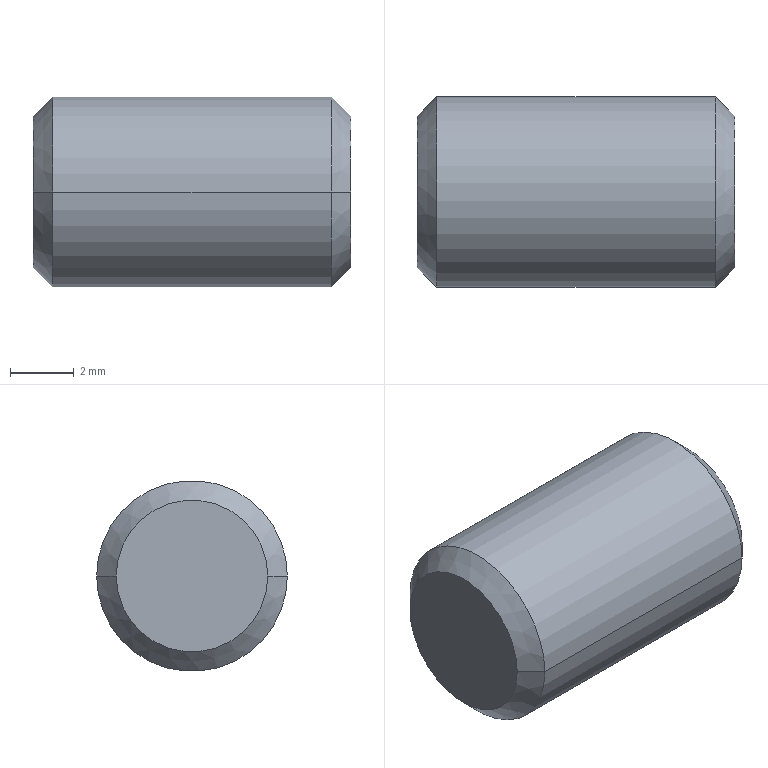Part | STEP file | KS B 1028 - Flat point M6x10 | 1 solid | 16 faces | box 10 x 6 x 6 mm | volume 245.798 mm3 | plane 8 | cone 6 | cylinder 2 | commonest cylinder face diameters 6 x2
STEP:
#1=CARTESIAN_POINT('',(0.,0.,0.));
#2=DIRECTION('',(0.,0.,1.));
#3=DIRECTION('',(1.,0.,0.));
#4=AXIS2_PLACEMENT_3D('',#1,#2,#3);
#5=CARTESIAN_POINT('',(0.,-2.387,0.));
#6=VERTEX_POINT('',#5);
#7=CARTESIAN_POINT('',(0.,2.387,0.));
#8=VERTEX_POINT('',#7);
#9=CARTESIAN_POINT('',(0.,0.,0.));
#10=DIRECTION('',(1.,0.,0.));
#11=DIRECTION('',(0.,-1.,0.));
#12=AXIS2_PLACEMENT_3D('',#9,#10,#11);
#13=CIRCLE('',#12,2.387);
#14=CARTESIAN_POINT('',(0.3067,0.,0.));
#15=DIRECTION('',(1.,0.,0.));
#16=DIRECTION('',(0.,-1.,0.));
#17=AXIS2_PLACEMENT_3D('',#14,#15,#16);
#18=CONICAL_SURFACE('',#17,2.693,0.7854);
#19=CARTESIAN_POINT('',(0.,-0.3067));
#20=DIRECTION('',(1.,0.));
#21=VECTOR('',#20,1.);
#22=LINE('',#19,#21);
#23=(GEOMETRIC_REPRESENTATION_CONTEXT(2)PARAMETRIC_REPRESENTATION_CONTEXT()REPRESENTATION_CONTEXT('',''));
#24=DEFINITIONAL_REPRESENTATION('',(#22),#23);
#25=PCURVE('',#18,#24);
#26=CARTESIAN_POINT('',(0.,1.5,0.));
#27=DIRECTION('',(-1.,0.,0.));
#28=DIRECTION('',(0.,1.,0.));
#29=AXIS2_PLACEMENT_3D('',#26,#27,#28);
#30=PLANE('',#29);
#31=CARTESIAN_POINT('',(-3.887,0.));
#32=CARTESIAN_POINT('',(-3.887,4.134));
#33=CARTESIAN_POINT('',(-0.3067,2.067));
#34=CARTESIAN_POINT('',(3.273,0.));
#35=CARTESIAN_POINT('',(-0.3067,-2.067));
#36=CARTESIAN_POINT('',(-3.887,-4.134));
#37=CARTESIAN_POINT('',(-3.887,0.));
#38=(BOUNDED_CURVE()B_SPLINE_CURVE(2,(#31,#32,#33,#34,#35,#36,#37),.UNSPECIFIED.,.T.,.F.)B_SPLINE_CURVE_WITH_KNOTS((1,2,2,2,2,1),(-2.094,0.,2.094,4.189,6.283,8.378),.UNSPECIFIED.)CURVE()GEOMETRIC_REPRESENTATION_ITEM()RATIONAL_B_SPLINE_CURVE((1.,0.5,1.,0.5,1.,0.5,1.))REPRESENTATION_ITEM(''));
#39=(GEOMETRIC_REPRESENTATION_CONTEXT(2)PARAMETRIC_REPRESENTATION_CONTEXT()REPRESENTATION_CONTEXT('',''));
#40=DEFINITIONAL_REPRESENTATION('',(#38),#39);
#41=PCURVE('',#30,#40);
#42=SURFACE_CURVE('',#13,(#25,#41),.PCURVE_S1.);
#43=EDGE_CURVE('',#6,#8,#42,.T.);
#44=ORIENTED_EDGE('',*,*,#43,.T.);
#45=CARTESIAN_POINT('',(0.6135,3.,0.));
#46=VERTEX_POINT('',#45);
#47=CARTESIAN_POINT('',(0.3067,2.693,0.));
#48=DIRECTION('',(0.7071,0.7071,0.));
#49=VECTOR('',#48,1.);
#50=LINE('',#47,#49);
#51=CARTESIAN_POINT('',(3.142,0.));
#52=DIRECTION('',(0.,1.));
#53=VECTOR('',#52,1.);
#54=LINE('',#51,#53);
#55=(GEOMETRIC_REPRESENTATION_CONTEXT(2)PARAMETRIC_REPRESENTATION_CONTEXT()REPRESENTATION_CONTEXT('',''));
#56=DEFINITIONAL_REPRESENTATION('',(#54),#55);
#57=PCURVE('',#18,#56);
#58=CARTESIAN_POINT('',(0.3067,0.,0.));
#59=DIRECTION('',(1.,0.,0.));
#60=DIRECTION('',(0.,-1.,0.));
#61=AXIS2_PLACEMENT_3D('',#58,#59,#60);
#62=CONICAL_SURFACE('',#61,2.693,0.7854);
#63=CARTESIAN_POINT('',(3.142,0.));
#64=DIRECTION('',(0.,1.));
#65=VECTOR('',#64,1.);
#66=LINE('',#63,#65);
#67=(GEOMETRIC_REPRESENTATION_CONTEXT(2)PARAMETRIC_REPRESENTATION_CONTEXT()REPRESENTATION_CONTEXT('',''));
#68=DEFINITIONAL_REPRESENTATION('',(#66),#67);
#69=PCURVE('',#62,#68);
#70=SURFACE_CURVE('',#50,(#57,#69),.PCURVE_S1.);
#71=EDGE_CURVE('',#8,#46,#70,.T.);
#72=ORIENTED_EDGE('',*,*,#71,.T.);
#73=CARTESIAN_POINT('',(0.6135,-3.,0.));
#74=VERTEX_POINT('',#73);
#75=CARTESIAN_POINT('',(0.6135,0.,0.));
#76=DIRECTION('',(-1.,0.,0.));
#77=DIRECTION('',(0.,-1.,0.));
#78=AXIS2_PLACEMENT_3D('',#75,#76,#77);
#79=CIRCLE('',#78,3.);
#80=CARTESIAN_POINT('',(6.283,0.3067));
#81=DIRECTION('',(-1.,0.));
#82=VECTOR('',#81,1.);
#83=LINE('',#80,#82);
#84=(GEOMETRIC_REPRESENTATION_CONTEXT(2)PARAMETRIC_REPRESENTATION_CONTEXT()REPRESENTATION_CONTEXT('',''));
#85=DEFINITIONAL_REPRESENTATION('',(#83),#84);
#86=PCURVE('',#18,#85);
#87=CARTESIAN_POINT('',(5.,0.,0.));
#88=DIRECTION('',(1.,0.,0.));
#89=DIRECTION('',(0.,1.,0.));
#90=AXIS2_PLACEMENT_3D('',#87,#88,#89);
#91=CYLINDRICAL_SURFACE('',#90,3.);
#92=CARTESIAN_POINT('',(9.425,-4.387));
#93=DIRECTION('',(-1.,0.));
#94=VECTOR('',#93,1.);
#95=LINE('',#92,#94);
#96=(GEOMETRIC_REPRESENTATION_CONTEXT(2)PARAMETRIC_REPRESENTATION_CONTEXT()REPRESENTATION_CONTEXT('',''));
#97=DEFINITIONAL_REPRESENTATION('',(#95),#96);
#98=PCURVE('',#91,#97);
#99=SURFACE_CURVE('',#79,(#86,#98),.PCURVE_S1.);
#100=EDGE_CURVE('',#46,#74,#99,.T.);
#101=ORIENTED_EDGE('',*,*,#100,.T.);
#102=CARTESIAN_POINT('',(0.3067,-2.693,0.));
#103=DIRECTION('',(0.7071,-0.7071,0.));
#104=VECTOR('',#103,1.);
#105=LINE('',#102,#104);
#106=CARTESIAN_POINT('',(0.,0.));
#107=DIRECTION('',(0.,1.));
#108=VECTOR('',#107,1.);
#109=LINE('',#106,#108);
#110=(GEOMETRIC_REPRESENTATION_CONTEXT(2)PARAMETRIC_REPRESENTATION_CONTEXT()REPRESENTATION_CONTEXT('',''));
#111=DEFINITIONAL_REPRESENTATION('',(#109),#110);
#112=PCURVE('',#18,#111);
#113=CARTESIAN_POINT('',(6.283,0.));
#114=DIRECTION('',(0.,1.));
#115=VECTOR('',#114,1.);
#116=LINE('',#113,#115);
#117=(GEOMETRIC_REPRESENTATION_CONTEXT(2)PARAMETRIC_REPRESENTATION_CONTEXT()REPRESENTATION_CONTEXT('',''));
#118=DEFINITIONAL_REPRESENTATION('',(#116),#117);
#119=PCURVE('',#62,#118);
#120=SURFACE_CURVE('',#105,(#112,#119),.PCURVE_S1.);
#121=EDGE_CURVE('',#6,#74,#120,.T.);
#122=ORIENTED_EDGE('',*,*,#121,.F.);
#123=EDGE_LOOP('',(#44,#72,#101,#122));
#124=FACE_BOUND('',#123,.T.);
#125=ADVANCED_FACE('',(#124),#18,.T.);
#126=CARTESIAN_POINT('',(0.6135,0.,0.));
#127=DIRECTION('',(-1.,0.,0.));
#128=DIRECTION('',(0.,-1.,0.));
#129=AXIS2_PLACEMENT_3D('',#126,#127,#128);
#130=CIRCLE('',#129,3.);
#131=CARTESIAN_POINT('',(5.,0.,0.));
#132=DIRECTION('',(1.,0.,0.));
#133=DIRECTION('',(0.,1.,0.));
#134=AXIS2_PLACEMENT_3D('',#131,#132,#133);
#135=CYLINDRICAL_SURFACE('',#134,3.);
#136=CARTESIAN_POINT('',(3.142,-4.387));
#137=DIRECTION('',(-1.,0.));
#138=VECTOR('',#137,1.);
#139=LINE('',#136,#138);
#140=(GEOMETRIC_REPRESENTATION_CONTEXT(2)PARAMETRIC_REPRESENTATION_CONTEXT()REPRESENTATION_CONTEXT('',''));
#141=DEFINITIONAL_REPRESENTATION('',(#139),#140);
#142=PCURVE('',#135,#141);
#143=CARTESIAN_POINT('',(6.283,0.3067));
#144=DIRECTION('',(-1.,0.));
#145=VECTOR('',#144,1.);
#146=LINE('',#143,#145);
#147=(GEOMETRIC_REPRESENTATION_CONTEXT(2)PARAMETRIC_REPRESENTATION_CONTEXT()REPRESENTATION_CONTEXT('',''));
#148=DEFINITIONAL_REPRESENTATION('',(#146),#147);
#149=PCURVE('',#62,#148);
#150=SURFACE_CURVE('',#130,(#142,#149),.PCURVE_S1.);
#151=EDGE_CURVE('',#74,#46,#150,.T.);
#152=ORIENTED_EDGE('',*,*,#151,.F.);
#153=CARTESIAN_POINT('',(9.387,-3.,0.));
#154=VERTEX_POINT('',#153);
#155=CARTESIAN_POINT('',(5.,-3.,0.));
#156=DIRECTION('',(1.,0.,0.));
#157=VECTOR('',#156,1.);
#158=LINE('',#155,#157);
#159=CARTESIAN_POINT('',(3.142,0.));
#160=DIRECTION('',(0.,1.));
#161=VECTOR('',#160,1.);
#162=LINE('',#159,#161);
#163=(GEOMETRIC_REPRESENTATION_CONTEXT(2)PARAMETRIC_REPRESENTATION_CONTEXT()REPRESENTATION_CONTEXT('',''));
#164=DEFINITIONAL_REPRESENTATION('',(#162),#163);
#165=PCURVE('',#135,#164);
#166=CARTESIAN_POINT('',(3.142,0.));
#167=DIRECTION('',(0.,1.));
#168=VECTOR('',#167,1.);
#169=LINE('',#166,#168);
#170=(GEOMETRIC_REPRESENTATION_CONTEXT(2)PARAMETRIC_REPRESENTATION_CONTEXT()REPRESENTATION_CONTEXT('',''));
#171=DEFINITIONAL_REPRESENTATION('',(#169),#170);
#172=PCURVE('',#91,#171);
#173=SURFACE_CURVE('',#158,(#165,#172),.PCURVE_S1.);
#174=EDGE_CURVE('',#74,#154,#173,.T.);
#175=ORIENTED_EDGE('',*,*,#174,.T.);
#176=CARTESIAN_POINT('',(9.387,3.,0.));
#177=VERTEX_POINT('',#176);
#178=CARTESIAN_POINT('',(9.387,0.,0.));
#179=DIRECTION('',(1.,0.,0.));
#180=DIRECTION('',(0.,-1.,0.));
#181=AXIS2_PLACEMENT_3D('',#178,#179,#180);
#182=CIRCLE('',#181,3.);
#183=CARTESIAN_POINT('',(-3.142,4.387));
#184=DIRECTION('',(1.,0.));
#185=VECTOR('',#184,1.);
#186=LINE('',#183,#185);
#187=(GEOMETRIC_REPRESENTATION_CONTEXT(2)PARAMETRIC_REPRESENTATION_CONTEXT()REPRESENTATION_CONTEXT('',''));
#188=DEFINITIONAL_REPRESENTATION('',(#186),#187);
#189=PCURVE('',#135,#188);
#190=CARTESIAN_POINT('',(9.693,0.,0.));
#191=DIRECTION('',(-1.,0.,0.));
#192=DIRECTION('',(0.,-1.,0.));
#193=AXIS2_PLACEMENT_3D('',#190,#191,#192);
#194=CONICAL_SURFACE('',#193,2.693,0.7854);
#195=CARTESIAN_POINT('',(6.283,0.3067));
#196=DIRECTION('',(-1.,0.));
#197=VECTOR('',#196,1.);
#198=LINE('',#195,#197);
#199=(GEOMETRIC_REPRESENTATION_CONTEXT(2)PARAMETRIC_REPRESENTATION_CONTEXT()REPRESENTATION_CONTEXT('',''));
#200=DEFINITIONAL_REPRESENTATION('',(#198),#199);
#201=PCURVE('',#194,#200);
#202=SURFACE_CURVE('',#182,(#189,#201),.PCURVE_S1.);
#203=EDGE_CURVE('',#177,#154,#202,.T.);
#204=ORIENTED_EDGE('',*,*,#203,.F.);
#205=CARTESIAN_POINT('',(5.,3.,0.));
#206=DIRECTION('',(1.,0.,0.));
#207=VECTOR('',#206,1.);
#208=LINE('',#205,#207);
#209=CARTESIAN_POINT('',(0.,0.));
#210=DIRECTION('',(0.,1.));
#211=VECTOR('',#210,1.);
#212=LINE('',#209,#211);
#213=(GEOMETRIC_REPRESENTATION_CONTEXT(2)PARAMETRIC_REPRESENTATION_CONTEXT()REPRESENTATION_CONTEXT('',''));
#214=DEFINITIONAL_REPRESENTATION('',(#212),#213);
#215=PCURVE('',#135,#214);
#216=CARTESIAN_POINT('',(6.283,0.));
#217=DIRECTION('',(0.,1.));
#218=VECTOR('',#217,1.);
#219=LINE('',#216,#218);
#220=(GEOMETRIC_REPRESENTATION_CONTEXT(2)PARAMETRIC_REPRESENTATION_CONTEXT()REPRESENTATION_CONTEXT('',''));
#221=DEFINITIONAL_REPRESENTATION('',(#219),#220);
#222=PCURVE('',#91,#221);
#223=SURFACE_CURVE('',#208,(#215,#222),.PCURVE_S1.);
#224=EDGE_CURVE('',#46,#177,#223,.T.);
#225=ORIENTED_EDGE('',*,*,#224,.F.);
#226=EDGE_LOOP('',(#152,#175,#204,#225));
#227=FACE_BOUND('',#226,.T.);
#228=ADVANCED_FACE('',(#227),#135,.T.);
#229=CARTESIAN_POINT('',(10.,-2.387,0.));
#230=VERTEX_POINT('',#229);
#231=CARTESIAN_POINT('',(10.,2.387,0.));
#232=VERTEX_POINT('',#231);
#233=CARTESIAN_POINT('',(10.,0.,0.));
#234=DIRECTION('',(-1.,0.,0.));
#235=DIRECTION('',(0.,-1.,0.));
#236=AXIS2_PLACEMENT_3D('',#233,#234,#235);
#237=CIRCLE('',#236,2.387);
#238=CARTESIAN_POINT('',(0.,-0.3067));
#239=DIRECTION('',(1.,0.));
#240=VECTOR('',#239,1.);
#241=LINE('',#238,#240);
#242=(GEOMETRIC_REPRESENTATION_CONTEXT(2)PARAMETRIC_REPRESENTATION_CONTEXT()REPRESENTATION_CONTEXT('',''));
#243=DEFINITIONAL_REPRESENTATION('',(#241),#242);
#244=PCURVE('',#194,#243);
#245=CARTESIAN_POINT('',(10.,0.,0.));
#246=DIRECTION('',(-1.,0.,0.));
#247=DIRECTION('',(0.,1.,0.));
#248=AXIS2_PLACEMENT_3D('',#245,#246,#247);
#249=PLANE('',#248);
#250=CARTESIAN_POINT('',(0.,0.));
#251=DIRECTION('',(-1.,0.));
#252=AXIS2_PLACEMENT_2D('',#250,#251);
#253=CIRCLE('',#252,2.387);
#254=(GEOMETRIC_REPRESENTATION_CONTEXT(2)PARAMETRIC_REPRESENTATION_CONTEXT()REPRESENTATION_CONTEXT('',''));
#255=DEFINITIONAL_REPRESENTATION('',(#253),#254);
#256=PCURVE('',#249,#255);
#257=SURFACE_CURVE('',#237,(#244,#256),.PCURVE_S1.);
#258=EDGE_CURVE('',#230,#232,#257,.T.);
#259=ORIENTED_EDGE('',*,*,#258,.T.);
#260=CARTESIAN_POINT('',(9.693,2.693,0.));
#261=DIRECTION('',(-0.7071,0.7071,0.));
#262=VECTOR('',#261,1.);
#263=LINE('',#260,#262);
#264=CARTESIAN_POINT('',(3.142,0.));
#265=DIRECTION('',(0.,1.));
#266=VECTOR('',#265,1.);
#267=LINE('',#264,#266);
#268=(GEOMETRIC_REPRESENTATION_CONTEXT(2)PARAMETRIC_REPRESENTATION_CONTEXT()REPRESENTATION_CONTEXT('',''));
#269=DEFINITIONAL_REPRESENTATION('',(#267),#268);
#270=PCURVE('',#194,#269);
#271=CARTESIAN_POINT('',(9.693,0.,0.));
#272=DIRECTION('',(-1.,0.,0.));
#273=DIRECTION('',(0.,-1.,0.));
#274=AXIS2_PLACEMENT_3D('',#271,#272,#273);
#275=CONICAL_SURFACE('',#274,2.693,0.7854);
#276=CARTESIAN_POINT('',(3.142,0.));
#277=DIRECTION('',(0.,1.));
#278=VECTOR('',#277,1.);
#279=LINE('',#276,#278);
#280=(GEOMETRIC_REPRESENTATION_CONTEXT(2)PARAMETRIC_REPRESENTATION_CONTEXT()REPRESENTATION_CONTEXT('',''));
#281=DEFINITIONAL_REPRESENTATION('',(#279),#280);
#282=PCURVE('',#275,#281);
#283=SURFACE_CURVE('',#263,(#270,#282),.PCURVE_S1.);
#284=EDGE_CURVE('',#232,#177,#283,.T.);
#285=ORIENTED_EDGE('',*,*,#284,.T.);
#286=ORIENTED_EDGE('',*,*,#203,.T.);
#287=CARTESIAN_POINT('',(9.693,-2.693,0.));
#288=DIRECTION('',(-0.7071,-0.7071,0.));
#289=VECTOR('',#288,1.);
#290=LINE('',#287,#289);
#291=CARTESIAN_POINT('',(0.,0.));
#292=DIRECTION('',(0.,1.));
#293=VECTOR('',#292,1.);
#294=LINE('',#291,#293);
#295=(GEOMETRIC_REPRESENTATION_CONTEXT(2)PARAMETRIC_REPRESENTATION_CONTEXT()REPRESENTATION_CONTEXT('',''));
#296=DEFINITIONAL_REPRESENTATION('',(#294),#295);
#297=PCURVE('',#194,#296);
#298=CARTESIAN_POINT('',(6.283,0.));
#299=DIRECTION('',(0.,1.));
#300=VECTOR('',#299,1.);
#301=LINE('',#298,#300);
#302=(GEOMETRIC_REPRESENTATION_CONTEXT(2)PARAMETRIC_REPRESENTATION_CONTEXT()REPRESENTATION_CONTEXT('',''));
#303=DEFINITIONAL_REPRESENTATION('',(#301),#302);
#304=PCURVE('',#275,#303);
#305=SURFACE_CURVE('',#290,(#297,#304),.PCURVE_S1.);
#306=EDGE_CURVE('',#230,#154,#305,.T.);
#307=ORIENTED_EDGE('',*,*,#306,.F.);
#308=EDGE_LOOP('',(#259,#285,#286,#307));
#309=FACE_BOUND('',#308,.T.);
#310=ADVANCED_FACE('',(#309),#194,.T.);
#311=CARTESIAN_POINT('',(6.5,1.5,-0.866));
#312=VERTEX_POINT('',#311);
#313=CARTESIAN_POINT('',(6.366,1.5,0.));
#314=VERTEX_POINT('',#313);
#315=CARTESIAN_POINT('',(6.5,1.5,-0.866));
#316=CARTESIAN_POINT('',(6.366,1.5,-0.4019));
#317=CARTESIAN_POINT('',(6.366,1.5,0.));
#318=(BOUNDED_CURVE()B_SPLINE_CURVE(2,(#315,#316,#317),.UNSPECIFIED.,.F.,.F.)B_SPLINE_CURVE_WITH_KNOTS((3,3),(0.,0.08763),.PIECEWISE_BEZIER_KNOTS.)CURVE()GEOMETRIC_REPRESENTATION_ITEM()RATIONAL_B_SPLINE_CURVE((1.,1.077,1.077))REPRESENTATION_ITEM(''));
#319=CARTESIAN_POINT('',(6.,0.,0.));
#320=DIRECTION('',(1.,0.,0.));
#321=DIRECTION('',(0.,1.,0.));
#322=AXIS2_PLACEMENT_3D('',#319,#320,#321);
#323=CONICAL_SURFACE('',#322,0.866,1.047);
#324=CARTESIAN_POINT('',(5.76,0.5));
#325=CARTESIAN_POINT('',(5.767,0.4956));
#326=CARTESIAN_POINT('',(5.782,0.4871));
#327=CARTESIAN_POINT('',(5.805,0.4752));
#328=CARTESIAN_POINT('',(5.828,0.4639));
#329=CARTESIAN_POINT('',(5.852,0.4534));
#330=CARTESIAN_POINT('',(5.875,0.4435));
#331=CARTESIAN_POINT('',(5.898,0.4343));
#332=CARTESIAN_POINT('',(5.922,0.4257));
#333=CARTESIAN_POINT('',(5.945,0.4178));
#334=CARTESIAN_POINT('',(5.969,0.4105));
#335=CARTESIAN_POINT('',(5.993,0.4037));
#336=CARTESIAN_POINT('',(6.017,0.3976));
#337=CARTESIAN_POINT('',(6.041,0.392));
#338=CARTESIAN_POINT('',(6.065,0.387));
#339=CARTESIAN_POINT('',(6.089,0.3825));
#340=CARTESIAN_POINT('',(6.113,0.3786));
#341=CARTESIAN_POINT('',(6.137,0.3752));
#342=CARTESIAN_POINT('',(6.162,0.3724));
#343=CARTESIAN_POINT('',(6.186,0.3701));
#344=CARTESIAN_POINT('',(6.21,0.3683));
#345=CARTESIAN_POINT('',(6.234,0.367));
#346=CARTESIAN_POINT('',(6.259,0.3662));
#347=CARTESIAN_POINT('',(6.275,0.366));
#348=CARTESIAN_POINT('',(6.283,0.366));
#349=B_SPLINE_CURVE_WITH_KNOTS('',3,(#324,#325,#326,#327,#328,#329,#330,#331,#332,#333,#334,#335,#336,#337,#338,#339,#340,#341,#342,#343,#344,#345,#346,#347,#348),.UNSPECIFIED.,.F.,.F.,(4,1,1,1,1,1,1,1,1,1,1,1,1,1,1,1,1,1,1,1,1,1,4),(0.,0.003983,0.007967,0.01195,0.01593,0.01992,0.0239,0.02788,0.03187,0.03585,0.03983,0.04382,0.0478,0.05178,0.05577,0.05975,0.06373,0.06772,0.0717,0.07568,0.07967,0.08365,0.08763),.QUASI_UNIFORM_KNOTS.);
#350=(GEOMETRIC_REPRESENTATION_CONTEXT(2)PARAMETRIC_REPRESENTATION_CONTEXT()REPRESENTATION_CONTEXT('',''));
#351=DEFINITIONAL_REPRESENTATION('',(#349),#350);
#352=PCURVE('',#323,#351);
#353=CARTESIAN_POINT('',(10.,1.5,-0.866));
#354=DIRECTION('',(0.,1.,0.));
#355=DIRECTION('',(0.,0.,-1.));
#356=AXIS2_PLACEMENT_3D('',#353,#354,#355);
#357=PLANE('',#356);
#358=CARTESIAN_POINT('',(0.,3.5));
#359=CARTESIAN_POINT('',(-0.4641,3.634));
#360=CARTESIAN_POINT('',(-0.866,3.634));
#361=(BOUNDED_CURVE()B_SPLINE_CURVE(2,(#358,#359,#360),.UNSPECIFIED.,.F.,.F.)B_SPLINE_CURVE_WITH_KNOTS((3,3),(0.,0.08763),.PIECEWISE_BEZIER_KNOTS.)CURVE()GEOMETRIC_REPRESENTATION_ITEM()RATIONAL_B_SPLINE_CURVE((1.,1.077,1.077))REPRESENTATION_ITEM(''));
#362=(GEOMETRIC_REPRESENTATION_CONTEXT(2)PARAMETRIC_REPRESENTATION_CONTEXT()REPRESENTATION_CONTEXT('',''));
#363=DEFINITIONAL_REPRESENTATION('',(#361),#362);
#364=PCURVE('',#357,#363);
#365=SURFACE_CURVE('',#318,(#352,#364),.PCURVE_S1.);
#366=EDGE_CURVE('',#312,#314,#365,.T.);
#367=ORIENTED_EDGE('',*,*,#366,.F.);
#368=CARTESIAN_POINT('',(6.5,0.,-1.732));
#369=VERTEX_POINT('',#368);
#370=CARTESIAN_POINT('',(6.5,0.,-1.732));
#371=CARTESIAN_POINT('',(6.25,0.75,-1.299));
#372=CARTESIAN_POINT('',(6.5,1.5,-0.866));
#373=(BOUNDED_CURVE()B_SPLINE_CURVE(2,(#370,#371,#372),.UNSPECIFIED.,.F.,.F.)B_SPLINE_CURVE_WITH_KNOTS((3,3),(0.,0.1753),.PIECEWISE_BEZIER_KNOTS.)CURVE()GEOMETRIC_REPRESENTATION_ITEM()RATIONAL_B_SPLINE_CURVE((1.,1.155,1.))REPRESENTATION_ITEM(''));
#374=CARTESIAN_POINT('',(4.712,0.5));
#375=CARTESIAN_POINT('',(4.728,0.4913));
#376=CARTESIAN_POINT('',(4.758,0.4748));
#377=CARTESIAN_POINT('',(4.804,0.453));
#378=CARTESIAN_POINT('',(4.851,0.434));
#379=CARTESIAN_POINT('',(4.898,0.4175));
#380=CARTESIAN_POINT('',(4.946,0.4034));
#381=CARTESIAN_POINT('',(4.994,0.3917));
#382=CARTESIAN_POINT('',(5.042,0.3823));
#383=CARTESIAN_POINT('',(5.09,0.375));
#384=CARTESIAN_POINT('',(5.139,0.3698));
#385=CARTESIAN_POINT('',(5.187,0.3667));
#386=CARTESIAN_POINT('',(5.236,0.3657));
#387=CARTESIAN_POINT('',(5.285,0.3667));
#388=CARTESIAN_POINT('',(5.333,0.3698));
#389=CARTESIAN_POINT('',(5.382,0.375));
#390=CARTESIAN_POINT('',(5.43,0.3823));
#391=CARTESIAN_POINT('',(5.478,0.3917));
#392=CARTESIAN_POINT('',(5.526,0.4034));
#393=CARTESIAN_POINT('',(5.574,0.4175));
#394=CARTESIAN_POINT('',(5.621,0.434));
#395=CARTESIAN_POINT('',(5.668,0.453));
#396=CARTESIAN_POINT('',(5.714,0.4748));
#397=CARTESIAN_POINT('',(5.744,0.4913));
#398=CARTESIAN_POINT('',(5.76,0.5));
#399=B_SPLINE_CURVE_WITH_KNOTS('',3,(#374,#375,#376,#377,#378,#379,#380,#381,#382,#383,#384,#385,#386,#387,#388,#389,#390,#391,#392,#393,#394,#395,#396,#397,#398),.UNSPECIFIED.,.F.,.F.,(4,1,1,1,1,1,1,1,1,1,1,1,1,1,1,1,1,1,1,1,1,1,4),(0.,0.007967,0.01593,0.0239,0.03187,0.03983,0.0478,0.05577,0.06373,0.0717,0.07967,0.08763,0.0956,0.1036,0.1115,0.1195,0.1275,0.1354,0.1434,0.1514,0.1593,0.1673,0.1753),.QUASI_UNIFORM_KNOTS.);
#400=(GEOMETRIC_REPRESENTATION_CONTEXT(2)PARAMETRIC_REPRESENTATION_CONTEXT()REPRESENTATION_CONTEXT('',''));
#401=DEFINITIONAL_REPRESENTATION('',(#399),#400);
#402=PCURVE('',#323,#401);
#403=CARTESIAN_POINT('',(10.,0.,-1.732));
#404=DIRECTION('',(0.,0.5,-0.866));
#405=DIRECTION('',(-1.,0.,0.));
#406=AXIS2_PLACEMENT_3D('',#403,#404,#405);
#407=PLANE('',#406);
#408=CARTESIAN_POINT('',(3.5,0.));
#409=CARTESIAN_POINT('',(3.75,0.866));
#410=CARTESIAN_POINT('',(3.5,1.732));
#411=(BOUNDED_CURVE()B_SPLINE_CURVE(2,(#408,#409,#410),.UNSPECIFIED.,.F.,.F.)B_SPLINE_CURVE_WITH_KNOTS((3,3),(0.,0.1753),.PIECEWISE_BEZIER_KNOTS.)CURVE()GEOMETRIC_REPRESENTATION_ITEM()RATIONAL_B_SPLINE_CURVE((1.,1.155,1.))REPRESENTATION_ITEM(''));
#412=(GEOMETRIC_REPRESENTATION_CONTEXT(2)PARAMETRIC_REPRESENTATION_CONTEXT()REPRESENTATION_CONTEXT('',''));
#413=DEFINITIONAL_REPRESENTATION('',(#411),#412);
#414=PCURVE('',#407,#413);
#415=SURFACE_CURVE('',#373,(#402,#414),.PCURVE_S1.);
#416=EDGE_CURVE('',#369,#312,#415,.T.);
#417=ORIENTED_EDGE('',*,*,#416,.F.);
#418=CARTESIAN_POINT('',(6.5,-1.5,-0.866));
#419=VERTEX_POINT('',#418);
#420=CARTESIAN_POINT('',(6.5,-1.5,-0.866));
#421=CARTESIAN_POINT('',(6.25,-0.75,-1.299));
#422=CARTESIAN_POINT('',(6.5,0.,-1.732));
#423=(BOUNDED_CURVE()B_SPLINE_CURVE(2,(#420,#421,#422),.UNSPECIFIED.,.F.,.F.)B_SPLINE_CURVE_WITH_KNOTS((3,3),(0.,0.1753),.PIECEWISE_BEZIER_KNOTS.)CURVE()GEOMETRIC_REPRESENTATION_ITEM()RATIONAL_B_SPLINE_CURVE((1.,1.155,1.))REPRESENTATION_ITEM(''));
#424=CARTESIAN_POINT('',(3.665,0.5));
#425=CARTESIAN_POINT('',(3.68,0.4913));
#426=CARTESIAN_POINT('',(3.711,0.4748));
#427=CARTESIAN_POINT('',(3.757,0.453));
#428=CARTESIAN_POINT('',(3.804,0.434));
#429=CARTESIAN_POINT('',(3.851,0.4175));
#430=CARTESIAN_POINT('',(3.898,0.4034));
#431=CARTESIAN_POINT('',(3.946,0.3917));
#432=CARTESIAN_POINT('',(3.994,0.3823));
#433=CARTESIAN_POINT('',(4.043,0.375));
#434=CARTESIAN_POINT('',(4.091,0.3698));
#435=CARTESIAN_POINT('',(4.14,0.3667));
#436=CARTESIAN_POINT('',(4.189,0.3657));
#437=CARTESIAN_POINT('',(4.238,0.3667));
#438=CARTESIAN_POINT('',(4.286,0.3698));
#439=CARTESIAN_POINT('',(4.335,0.375));
#440=CARTESIAN_POINT('',(4.383,0.3823));
#441=CARTESIAN_POINT('',(4.431,0.3917));
#442=CARTESIAN_POINT('',(4.479,0.4034));
#443=CARTESIAN_POINT('',(4.527,0.4175));
#444=CARTESIAN_POINT('',(4.574,0.434));
#445=CARTESIAN_POINT('',(4.621,0.453));
#446=CARTESIAN_POINT('',(4.667,0.4748));
#447=CARTESIAN_POINT('',(4.697,0.4913));
#448=CARTESIAN_POINT('',(4.712,0.5));
#449=B_SPLINE_CURVE_WITH_KNOTS('',3,(#424,#425,#426,#427,#428,#429,#430,#431,#432,#433,#434,#435,#436,#437,#438,#439,#440,#441,#442,#443,#444,#445,#446,#447,#448),.UNSPECIFIED.,.F.,.F.,(4,1,1,1,1,1,1,1,1,1,1,1,1,1,1,1,1,1,1,1,1,1,4),(0.,0.007967,0.01593,0.0239,0.03187,0.03983,0.0478,0.05577,0.06373,0.0717,0.07967,0.08763,0.0956,0.1036,0.1115,0.1195,0.1275,0.1354,0.1434,0.1514,0.1593,0.1673,0.1753),.QUASI_UNIFORM_KNOTS.);
#450=(GEOMETRIC_REPRESENTATION_CONTEXT(2)PARAMETRIC_REPRESENTATION_CONTEXT()REPRESENTATION_CONTEXT('',''));
#451=DEFINITIONAL_REPRESENTATION('',(#449),#450);
#452=PCURVE('',#323,#451);
#453=CARTESIAN_POINT('',(10.,-1.5,-0.866));
#454=DIRECTION('',(0.,-0.5,-0.866));
#455=DIRECTION('',(0.,-0.866,0.5));
#456=AXIS2_PLACEMENT_3D('',#453,#454,#455);
#457=PLANE('',#456);
#458=CARTESIAN_POINT('',(0.,3.5));
#459=CARTESIAN_POINT('',(-0.866,3.75));
#460=CARTESIAN_POINT('',(-1.732,3.5));
#461=(BOUNDED_CURVE()B_SPLINE_CURVE(2,(#458,#459,#460),.UNSPECIFIED.,.F.,.F.)B_SPLINE_CURVE_WITH_KNOTS((3,3),(0.,0.1753),.PIECEWISE_BEZIER_KNOTS.)CURVE()GEOMETRIC_REPRESENTATION_ITEM()RATIONAL_B_SPLINE_CURVE((1.,1.155,1.))REPRESENTATION_ITEM(''));
#462=(GEOMETRIC_REPRESENTATION_CONTEXT(2)PARAMETRIC_REPRESENTATION_CONTEXT()REPRESENTATION_CONTEXT('',''));
#463=DEFINITIONAL_REPRESENTATION('',(#461),#462);
#464=PCURVE('',#457,#463);
#465=SURFACE_CURVE('',#423,(#452,#464),.PCURVE_S1.);
#466=EDGE_CURVE('',#419,#369,#465,.T.);
#467=ORIENTED_EDGE('',*,*,#466,.F.);
#468=CARTESIAN_POINT('',(6.366,-1.5,0.));
#469=VERTEX_POINT('',#468);
#470=CARTESIAN_POINT('',(6.366,-1.5,0.));
#471=CARTESIAN_POINT('',(6.366,-1.5,-0.4019));
#472=CARTESIAN_POINT('',(6.5,-1.5,-0.866));
#473=(BOUNDED_CURVE()B_SPLINE_CURVE(2,(#470,#471,#472),.UNSPECIFIED.,.F.,.F.)B_SPLINE_CURVE_WITH_KNOTS((3,3),(0.08763,0.1753),.PIECEWISE_BEZIER_KNOTS.)CURVE()GEOMETRIC_REPRESENTATION_ITEM()RATIONAL_B_SPLINE_CURVE((1.077,1.077,1.))REPRESENTATION_ITEM(''));
#474=CARTESIAN_POINT('',(3.142,0.366));
#475=CARTESIAN_POINT('',(3.15,0.366));
#476=CARTESIAN_POINT('',(3.166,0.3662));
#477=CARTESIAN_POINT('',(3.19,0.367));
#478=CARTESIAN_POINT('',(3.215,0.3683));
#479=CARTESIAN_POINT('',(3.239,0.3701));
#480=CARTESIAN_POINT('',(3.263,0.3724));
#481=CARTESIAN_POINT('',(3.287,0.3752));
#482=CARTESIAN_POINT('',(3.312,0.3786));
#483=CARTESIAN_POINT('',(3.336,0.3825));
#484=CARTESIAN_POINT('',(3.36,0.387));
#485=CARTESIAN_POINT('',(3.384,0.392));
#486=CARTESIAN_POINT('',(3.408,0.3976));
#487=CARTESIAN_POINT('',(3.432,0.4037));
#488=CARTESIAN_POINT('',(3.456,0.4105));
#489=CARTESIAN_POINT('',(3.479,0.4178));
#490=CARTESIAN_POINT('',(3.503,0.4257));
#491=CARTESIAN_POINT('',(3.527,0.4343));
#492=CARTESIAN_POINT('',(3.55,0.4435));
#493=CARTESIAN_POINT('',(3.573,0.4534));
#494=CARTESIAN_POINT('',(3.596,0.4639));
#495=CARTESIAN_POINT('',(3.619,0.4752));
#496=CARTESIAN_POINT('',(3.642,0.4871));
#497=CARTESIAN_POINT('',(3.658,0.4956));
#498=CARTESIAN_POINT('',(3.665,0.5));
#499=B_SPLINE_CURVE_WITH_KNOTS('',3,(#474,#475,#476,#477,#478,#479,#480,#481,#482,#483,#484,#485,#486,#487,#488,#489,#490,#491,#492,#493,#494,#495,#496,#497,#498),.UNSPECIFIED.,.F.,.F.,(4,1,1,1,1,1,1,1,1,1,1,1,1,1,1,1,1,1,1,1,1,1,4),(0.08763,0.09162,0.0956,0.09958,0.1036,0.1075,0.1115,0.1155,0.1195,0.1235,0.1275,0.1314,0.1354,0.1394,0.1434,0.1474,0.1514,0.1553,0.1593,0.1633,0.1673,0.1713,0.1753),.QUASI_UNIFORM_KNOTS.);
#500=(GEOMETRIC_REPRESENTATION_CONTEXT(2)PARAMETRIC_REPRESENTATION_CONTEXT()REPRESENTATION_CONTEXT('',''));
#501=DEFINITIONAL_REPRESENTATION('',(#499),#500);
#502=PCURVE('',#323,#501);
#503=CARTESIAN_POINT('',(10.,-1.5,0.866));
#504=DIRECTION('',(0.,-1.,0.));
#505=DIRECTION('',(0.,0.,-1.));
#506=AXIS2_PLACEMENT_3D('',#503,#504,#505);
#507=PLANE('',#506);
#508=CARTESIAN_POINT('',(0.866,-3.634));
#509=CARTESIAN_POINT('',(1.268,-3.634));
#510=CARTESIAN_POINT('',(1.732,-3.5));
#511=(BOUNDED_CURVE()B_SPLINE_CURVE(2,(#508,#509,#510),.UNSPECIFIED.,.F.,.F.)B_SPLINE_CURVE_WITH_KNOTS((3,3),(0.08763,0.1753),.PIECEWISE_BEZIER_KNOTS.)CURVE()GEOMETRIC_REPRESENTATION_ITEM()RATIONAL_B_SPLINE_CURVE((1.077,1.077,1.))REPRESENTATION_ITEM(''));
#512=(GEOMETRIC_REPRESENTATION_CONTEXT(2)PARAMETRIC_REPRESENTATION_CONTEXT()REPRESENTATION_CONTEXT('',''));
#513=DEFINITIONAL_REPRESENTATION('',(#511),#512);
#514=PCURVE('',#507,#513);
#515=SURFACE_CURVE('',#473,(#502,#514),.PCURVE_S1.);
#516=EDGE_CURVE('',#469,#419,#515,.T.);
#517=ORIENTED_EDGE('',*,*,#516,.F.);
#518=CARTESIAN_POINT('',(5.5,0.,0.));
#519=VERTEX_POINT('',#518);
#520=CARTESIAN_POINT('',(6.,-0.866,0.));
#521=DIRECTION('',(0.5,-0.866,0.));
#522=VECTOR('',#521,1.);
#523=LINE('',#520,#522);
#524=CARTESIAN_POINT('',(3.142,0.));
#525=DIRECTION('',(0.,1.));
#526=VECTOR('',#525,1.);
#527=LINE('',#524,#526);
#528=(GEOMETRIC_REPRESENTATION_CONTEXT(2)PARAMETRIC_REPRESENTATION_CONTEXT()REPRESENTATION_CONTEXT('',''));
#529=DEFINITIONAL_REPRESENTATION('',(#527),#528);
#530=PCURVE('',#323,#529);
#531=CARTESIAN_POINT('',(6.,0.,0.));
#532=DIRECTION('',(1.,0.,0.));
#533=DIRECTION('',(0.,1.,0.));
#534=AXIS2_PLACEMENT_3D('',#531,#532,#533);
#535=CONICAL_SURFACE('',#534,0.866,1.047);
#536=CARTESIAN_POINT('',(3.142,0.));
#537=DIRECTION('',(0.,1.));
#538=VECTOR('',#537,1.);
#539=LINE('',#536,#538);
#540=(GEOMETRIC_REPRESENTATION_CONTEXT(2)PARAMETRIC_REPRESENTATION_CONTEXT()REPRESENTATION_CONTEXT('',''));
#541=DEFINITIONAL_REPRESENTATION('',(#539),#540);
#542=PCURVE('',#535,#541);
#543=SURFACE_CURVE('',#523,(#530,#542),.PCURVE_S1.);
#544=EDGE_CURVE('',#519,#469,#543,.T.);
#545=ORIENTED_EDGE('',*,*,#544,.F.);
#546=CARTESIAN_POINT('',(6.,0.866,0.));
#547=DIRECTION('',(0.5,0.866,0.));
#548=VECTOR('',#547,1.);
#549=LINE('',#546,#548);
#550=CARTESIAN_POINT('',(6.283,0.));
#551=DIRECTION('',(0.,1.));
#552=VECTOR('',#551,1.);
#553=LINE('',#550,#552);
#554=(GEOMETRIC_REPRESENTATION_CONTEXT(2)PARAMETRIC_REPRESENTATION_CONTEXT()REPRESENTATION_CONTEXT('',''));
#555=DEFINITIONAL_REPRESENTATION('',(#553),#554);
#556=PCURVE('',#323,#555);
#557=CARTESIAN_POINT('',(0.,0.));
#558=DIRECTION('',(0.,1.));
#559=VECTOR('',#558,1.);
#560=LINE('',#557,#559);
#561=(GEOMETRIC_REPRESENTATION_CONTEXT(2)PARAMETRIC_REPRESENTATION_CONTEXT()REPRESENTATION_CONTEXT('',''));
#562=DEFINITIONAL_REPRESENTATION('',(#560),#561);
#563=PCURVE('',#535,#562);
#564=SURFACE_CURVE('',#549,(#556,#563),.PCURVE_S1.);
#565=EDGE_CURVE('',#519,#314,#564,.T.);
#566=ORIENTED_EDGE('',*,*,#565,.T.);
#567=EDGE_LOOP('',(#367,#417,#467,#517,#545,#566));
#568=FACE_BOUND('',#567,.F.);
#569=ADVANCED_FACE('',(#568),#323,.F.);
#570=CARTESIAN_POINT('',(6.5,-1.5,0.866));
#571=VERTEX_POINT('',#570);
#572=CARTESIAN_POINT('',(6.5,-1.5,0.866));
#573=CARTESIAN_POINT('',(6.366,-1.5,0.4019));
#574=CARTESIAN_POINT('',(6.366,-1.5,0.));
#575=(BOUNDED_CURVE()B_SPLINE_CURVE(2,(#572,#573,#574),.UNSPECIFIED.,.F.,.F.)B_SPLINE_CURVE_WITH_KNOTS((3,3),(0.,0.08763),.PIECEWISE_BEZIER_KNOTS.)CURVE()GEOMETRIC_REPRESENTATION_ITEM()RATIONAL_B_SPLINE_CURVE((1.,1.077,1.077))REPRESENTATION_ITEM(''));
#576=CARTESIAN_POINT('',(2.618,0.5));
#577=CARTESIAN_POINT('',(2.626,0.4956));
#578=CARTESIAN_POINT('',(2.641,0.4871));
#579=CARTESIAN_POINT('',(2.664,0.4752));
#580=CARTESIAN_POINT('',(2.687,0.4639));
#581=CARTESIAN_POINT('',(2.71,0.4534));
#582=CARTESIAN_POINT('',(2.733,0.4435));
#583=CARTESIAN_POINT('',(2.757,0.4343));
#584=CARTESIAN_POINT('',(2.78,0.4257));
#585=CARTESIAN_POINT('',(2.804,0.4178));
#586=CARTESIAN_POINT('',(2.828,0.4105));
#587=CARTESIAN_POINT('',(2.851,0.4037));
#588=CARTESIAN_POINT('',(2.875,0.3976));
#589=CARTESIAN_POINT('',(2.899,0.392));
#590=CARTESIAN_POINT('',(2.923,0.387));
#591=CARTESIAN_POINT('',(2.947,0.3825));
#592=CARTESIAN_POINT('',(2.971,0.3786));
#593=CARTESIAN_POINT('',(2.996,0.3752));
#594=CARTESIAN_POINT('',(3.02,0.3724));
#595=CARTESIAN_POINT('',(3.044,0.3701));
#596=CARTESIAN_POINT('',(3.069,0.3683));
#597=CARTESIAN_POINT('',(3.093,0.367));
#598=CARTESIAN_POINT('',(3.117,0.3662));
#599=CARTESIAN_POINT('',(3.133,0.366));
#600=CARTESIAN_POINT('',(3.142,0.366));
#601=B_SPLINE_CURVE_WITH_KNOTS('',3,(#576,#577,#578,#579,#580,#581,#582,#583,#584,#585,#586,#587,#588,#589,#590,#591,#592,#593,#594,#595,#596,#597,#598,#599,#600),.UNSPECIFIED.,.F.,.F.,(4,1,1,1,1,1,1,1,1,1,1,1,1,1,1,1,1,1,1,1,1,1,4),(0.,0.003983,0.007967,0.01195,0.01593,0.01992,0.0239,0.02788,0.03187,0.03585,0.03983,0.04382,0.0478,0.05178,0.05577,0.05975,0.06373,0.06772,0.0717,0.07568,0.07967,0.08365,0.08763),.QUASI_UNIFORM_KNOTS.);
#602=(GEOMETRIC_REPRESENTATION_CONTEXT(2)PARAMETRIC_REPRESENTATION_CONTEXT()REPRESENTATION_CONTEXT('',''));
#603=DEFINITIONAL_REPRESENTATION('',(#601),#602);
#604=PCURVE('',#535,#603);
#605=CARTESIAN_POINT('',(0.,-3.5));
#606=CARTESIAN_POINT('',(0.4641,-3.634));
#607=CARTESIAN_POINT('',(0.866,-3.634));
#608=(BOUNDED_CURVE()B_SPLINE_CURVE(2,(#605,#606,#607),.UNSPECIFIED.,.F.,.F.)B_SPLINE_CURVE_WITH_KNOTS((3,3),(0.,0.08763),.PIECEWISE_BEZIER_KNOTS.)CURVE()GEOMETRIC_REPRESENTATION_ITEM()RATIONAL_B_SPLINE_CURVE((1.,1.077,1.077))REPRESENTATION_ITEM(''));
#609=(GEOMETRIC_REPRESENTATION_CONTEXT(2)PARAMETRIC_REPRESENTATION_CONTEXT()REPRESENTATION_CONTEXT('',''));
#610=DEFINITIONAL_REPRESENTATION('',(#608),#609);
#611=PCURVE('',#507,#610);
#612=SURFACE_CURVE('',#575,(#604,#611),.PCURVE_S1.);
#613=EDGE_CURVE('',#571,#469,#612,.T.);
#614=ORIENTED_EDGE('',*,*,#613,.F.);
#615=CARTESIAN_POINT('',(6.5,0.,1.732));
#616=VERTEX_POINT('',#615);
#617=CARTESIAN_POINT('',(6.5,0.,1.732));
#618=CARTESIAN_POINT('',(6.25,-0.75,1.299));
#619=CARTESIAN_POINT('',(6.5,-1.5,0.866));
#620=(BOUNDED_CURVE()B_SPLINE_CURVE(2,(#617,#618,#619),.UNSPECIFIED.,.F.,.F.)B_SPLINE_CURVE_WITH_KNOTS((3,3),(0.,0.1753),.PIECEWISE_BEZIER_KNOTS.)CURVE()GEOMETRIC_REPRESENTATION_ITEM()RATIONAL_B_SPLINE_CURVE((1.,1.155,1.))REPRESENTATION_ITEM(''));
#621=CARTESIAN_POINT('',(1.571,0.5));
#622=CARTESIAN_POINT('',(1.586,0.4913));
#623=CARTESIAN_POINT('',(1.616,0.4748));
#624=CARTESIAN_POINT('',(1.663,0.453));
#625=CARTESIAN_POINT('',(1.709,0.434));
#626=CARTESIAN_POINT('',(1.757,0.4175));
#627=CARTESIAN_POINT('',(1.804,0.4034));
#628=CARTESIAN_POINT('',(1.852,0.3917));
#629=CARTESIAN_POINT('',(1.9,0.3823));
#630=CARTESIAN_POINT('',(1.948,0.375));
#631=CARTESIAN_POINT('',(1.997,0.3698));
#632=CARTESIAN_POINT('',(2.046,0.3667));
#633=CARTESIAN_POINT('',(2.094,0.3657));
#634=CARTESIAN_POINT('',(2.143,0.3667));
#635=CARTESIAN_POINT('',(2.192,0.3698));
#636=CARTESIAN_POINT('',(2.24,0.375));
#637=CARTESIAN_POINT('',(2.289,0.3823));
#638=CARTESIAN_POINT('',(2.337,0.3917));
#639=CARTESIAN_POINT('',(2.385,0.4034));
#640=CARTESIAN_POINT('',(2.432,0.4175));
#641=CARTESIAN_POINT('',(2.479,0.434));
#642=CARTESIAN_POINT('',(2.526,0.453));
#643=CARTESIAN_POINT('',(2.572,0.4748));
#644=CARTESIAN_POINT('',(2.603,0.4913));
#645=CARTESIAN_POINT('',(2.618,0.5));
#646=B_SPLINE_CURVE_WITH_KNOTS('',3,(#621,#622,#623,#624,#625,#626,#627,#628,#629,#630,#631,#632,#633,#634,#635,#636,#637,#638,#639,#640,#641,#642,#643,#644,#645),.UNSPECIFIED.,.F.,.F.,(4,1,1,1,1,1,1,1,1,1,1,1,1,1,1,1,1,1,1,1,1,1,4),(0.,0.007967,0.01593,0.0239,0.03187,0.03983,0.0478,0.05577,0.06373,0.0717,0.07967,0.08763,0.0956,0.1036,0.1115,0.1195,0.1275,0.1354,0.1434,0.1514,0.1593,0.1673,0.1753),.QUASI_UNIFORM_KNOTS.);
#647=(GEOMETRIC_REPRESENTATION_CONTEXT(2)PARAMETRIC_REPRESENTATION_CONTEXT()REPRESENTATION_CONTEXT('',''));
#648=DEFINITIONAL_REPRESENTATION('',(#646),#647);
#649=PCURVE('',#535,#648);
#650=CARTESIAN_POINT('',(10.,0.,1.732));
#651=DIRECTION('',(0.,-0.5,0.866));
#652=DIRECTION('',(-1.,0.,0.));
#653=AXIS2_PLACEMENT_3D('',#650,#651,#652);
#654=PLANE('',#653);
#655=CARTESIAN_POINT('',(3.5,0.));
#656=CARTESIAN_POINT('',(3.75,0.866));
#657=CARTESIAN_POINT('',(3.5,1.732));
#658=(BOUNDED_CURVE()B_SPLINE_CURVE(2,(#655,#656,#657),.UNSPECIFIED.,.F.,.F.)B_SPLINE_CURVE_WITH_KNOTS((3,3),(0.,0.1753),.PIECEWISE_BEZIER_KNOTS.)CURVE()GEOMETRIC_REPRESENTATION_ITEM()RATIONAL_B_SPLINE_CURVE((1.,1.155,1.))REPRESENTATION_ITEM(''));
#659=(GEOMETRIC_REPRESENTATION_CONTEXT(2)PARAMETRIC_REPRESENTATION_CONTEXT()REPRESENTATION_CONTEXT('',''));
#660=DEFINITIONAL_REPRESENTATION('',(#658),#659);
#661=PCURVE('',#654,#660);
#662=SURFACE_CURVE('',#620,(#649,#661),.PCURVE_S1.);
#663=EDGE_CURVE('',#616,#571,#662,.T.);
#664=ORIENTED_EDGE('',*,*,#663,.F.);
#665=CARTESIAN_POINT('',(6.5,1.5,0.866));
#666=VERTEX_POINT('',#665);
#667=CARTESIAN_POINT('',(6.5,1.5,0.866));
#668=CARTESIAN_POINT('',(6.25,0.75,1.299));
#669=CARTESIAN_POINT('',(6.5,0.,1.732));
#670=(BOUNDED_CURVE()B_SPLINE_CURVE(2,(#667,#668,#669),.UNSPECIFIED.,.F.,.F.)B_SPLINE_CURVE_WITH_KNOTS((3,3),(0.,0.1753),.PIECEWISE_BEZIER_KNOTS.)CURVE()GEOMETRIC_REPRESENTATION_ITEM()RATIONAL_B_SPLINE_CURVE((1.,1.155,1.))REPRESENTATION_ITEM(''));
#671=CARTESIAN_POINT('',(0.5236,0.5));
#672=CARTESIAN_POINT('',(0.5388,0.4913));
#673=CARTESIAN_POINT('',(0.5692,0.4748));
#674=CARTESIAN_POINT('',(0.6155,0.453));
#675=CARTESIAN_POINT('',(0.6622,0.434));
#676=CARTESIAN_POINT('',(0.7094,0.4175));
#677=CARTESIAN_POINT('',(0.7569,0.4034));
#678=CARTESIAN_POINT('',(0.8048,0.3917));
#679=CARTESIAN_POINT('',(0.8529,0.3823));
#680=CARTESIAN_POINT('',(0.9013,0.375));
#681=CARTESIAN_POINT('',(0.9498,0.3698));
#682=CARTESIAN_POINT('',(0.9985,0.3667));
#683=CARTESIAN_POINT('',(1.047,0.3657));
#684=CARTESIAN_POINT('',(1.096,0.3667));
#685=CARTESIAN_POINT('',(1.145,0.3698));
#686=CARTESIAN_POINT('',(1.193,0.375));
#687=CARTESIAN_POINT('',(1.241,0.3823));
#688=CARTESIAN_POINT('',(1.29,0.3917));
#689=CARTESIAN_POINT('',(1.338,0.4034));
#690=CARTESIAN_POINT('',(1.385,0.4175));
#691=CARTESIAN_POINT('',(1.432,0.434));
#692=CARTESIAN_POINT('',(1.479,0.453));
#693=CARTESIAN_POINT('',(1.525,0.4748));
#694=CARTESIAN_POINT('',(1.556,0.4913));
#695=CARTESIAN_POINT('',(1.571,0.5));
#696=B_SPLINE_CURVE_WITH_KNOTS('',3,(#671,#672,#673,#674,#675,#676,#677,#678,#679,#680,#681,#682,#683,#684,#685,#686,#687,#688,#689,#690,#691,#692,#693,#694,#695),.UNSPECIFIED.,.F.,.F.,(4,1,1,1,1,1,1,1,1,1,1,1,1,1,1,1,1,1,1,1,1,1,4),(0.,0.007967,0.01593,0.0239,0.03187,0.03983,0.0478,0.05577,0.06373,0.0717,0.07967,0.08763,0.0956,0.1036,0.1115,0.1195,0.1275,0.1354,0.1434,0.1514,0.1593,0.1673,0.1753),.QUASI_UNIFORM_KNOTS.);
#697=(GEOMETRIC_REPRESENTATION_CONTEXT(2)PARAMETRIC_REPRESENTATION_CONTEXT()REPRESENTATION_CONTEXT('',''));
#698=DEFINITIONAL_REPRESENTATION('',(#696),#697);
#699=PCURVE('',#535,#698);
#700=CARTESIAN_POINT('',(10.,1.5,0.866));
#701=DIRECTION('',(0.,0.5,0.866));
#702=DIRECTION('',(1.,0.,0.));
#703=AXIS2_PLACEMENT_3D('',#700,#701,#702);
#704=PLANE('',#703);
#705=CARTESIAN_POINT('',(-3.5,0.));
#706=CARTESIAN_POINT('',(-3.75,-0.866));
#707=CARTESIAN_POINT('',(-3.5,-1.732));
#708=(BOUNDED_CURVE()B_SPLINE_CURVE(2,(#705,#706,#707),.UNSPECIFIED.,.F.,.F.)B_SPLINE_CURVE_WITH_KNOTS((3,3),(0.,0.1753),.PIECEWISE_BEZIER_KNOTS.)CURVE()GEOMETRIC_REPRESENTATION_ITEM()RATIONAL_B_SPLINE_CURVE((1.,1.155,1.))REPRESENTATION_ITEM(''));
#709=(GEOMETRIC_REPRESENTATION_CONTEXT(2)PARAMETRIC_REPRESENTATION_CONTEXT()REPRESENTATION_CONTEXT('',''));
#710=DEFINITIONAL_REPRESENTATION('',(#708),#709);
#711=PCURVE('',#704,#710);
#712=SURFACE_CURVE('',#670,(#699,#711),.PCURVE_S1.);
#713=EDGE_CURVE('',#666,#616,#712,.T.);
#714=ORIENTED_EDGE('',*,*,#713,.F.);
#715=CARTESIAN_POINT('',(6.366,1.5,0.));
#716=CARTESIAN_POINT('',(6.366,1.5,0.4019));
#717=CARTESIAN_POINT('',(6.5,1.5,0.866));
#718=(BOUNDED_CURVE()B_SPLINE_CURVE(2,(#715,#716,#717),.UNSPECIFIED.,.F.,.F.)B_SPLINE_CURVE_WITH_KNOTS((3,3),(0.08763,0.1753),.PIECEWISE_BEZIER_KNOTS.)CURVE()GEOMETRIC_REPRESENTATION_ITEM()RATIONAL_B_SPLINE_CURVE((1.077,1.077,1.))REPRESENTATION_ITEM(''));
#719=CARTESIAN_POINT('',(0.,0.366));
#720=CARTESIAN_POINT('',(0.00812,0.366));
#721=CARTESIAN_POINT('',(0.02436,0.3662));
#722=CARTESIAN_POINT('',(0.04871,0.367));
#723=CARTESIAN_POINT('',(0.07305,0.3683));
#724=CARTESIAN_POINT('',(0.09736,0.3701));
#725=CARTESIAN_POINT('',(0.1217,0.3724));
#726=CARTESIAN_POINT('',(0.1459,0.3752));
#727=CARTESIAN_POINT('',(0.1701,0.3786));
#728=CARTESIAN_POINT('',(0.1943,0.3825));
#729=CARTESIAN_POINT('',(0.2184,0.387));
#730=CARTESIAN_POINT('',(0.2424,0.392));
#731=CARTESIAN_POINT('',(0.2664,0.3976));
#732=CARTESIAN_POINT('',(0.2903,0.4037));
#733=CARTESIAN_POINT('',(0.3141,0.4105));
#734=CARTESIAN_POINT('',(0.3378,0.4178));
#735=CARTESIAN_POINT('',(0.3614,0.4257));
#736=CARTESIAN_POINT('',(0.3849,0.4343));
#737=CARTESIAN_POINT('',(0.4084,0.4435));
#738=CARTESIAN_POINT('',(0.4317,0.4534));
#739=CARTESIAN_POINT('',(0.4548,0.4639));
#740=CARTESIAN_POINT('',(0.4779,0.4752));
#741=CARTESIAN_POINT('',(0.5008,0.4871));
#742=CARTESIAN_POINT('',(0.516,0.4956));
#743=CARTESIAN_POINT('',(0.5236,0.5));
#744=B_SPLINE_CURVE_WITH_KNOTS('',3,(#719,#720,#721,#722,#723,#724,#725,#726,#727,#728,#729,#730,#731,#732,#733,#734,#735,#736,#737,#738,#739,#740,#741,#742,#743),.UNSPECIFIED.,.F.,.F.,(4,1,1,1,1,1,1,1,1,1,1,1,1,1,1,1,1,1,1,1,1,1,4),(0.08763,0.09162,0.0956,0.09958,0.1036,0.1075,0.1115,0.1155,0.1195,0.1235,0.1275,0.1314,0.1354,0.1394,0.1434,0.1474,0.1514,0.1553,0.1593,0.1633,0.1673,0.1713,0.1753),.QUASI_UNIFORM_KNOTS.);
#745=(GEOMETRIC_REPRESENTATION_CONTEXT(2)PARAMETRIC_REPRESENTATION_CONTEXT()REPRESENTATION_CONTEXT('',''));
#746=DEFINITIONAL_REPRESENTATION('',(#744),#745);
#747=PCURVE('',#535,#746);
#748=CARTESIAN_POINT('',(-0.866,3.634));
#749=CARTESIAN_POINT('',(-1.268,3.634));
#750=CARTESIAN_POINT('',(-1.732,3.5));
#751=(BOUNDED_CURVE()B_SPLINE_CURVE(2,(#748,#749,#750),.UNSPECIFIED.,.F.,.F.)B_SPLINE_CURVE_WITH_KNOTS((3,3),(0.08763,0.1753),.PIECEWISE_BEZIER_KNOTS.)CURVE()GEOMETRIC_REPRESENTATION_ITEM()RATIONAL_B_SPLINE_CURVE((1.077,1.077,1.))REPRESENTATION_ITEM(''));
#752=(GEOMETRIC_REPRESENTATION_CONTEXT(2)PARAMETRIC_REPRESENTATION_CONTEXT()REPRESENTATION_CONTEXT('',''));
#753=DEFINITIONAL_REPRESENTATION('',(#751),#752);
#754=PCURVE('',#357,#753);
#755=SURFACE_CURVE('',#718,(#747,#754),.PCURVE_S1.);
#756=EDGE_CURVE('',#314,#666,#755,.T.);
#757=ORIENTED_EDGE('',*,*,#756,.F.);
#758=ORIENTED_EDGE('',*,*,#565,.F.);
#759=ORIENTED_EDGE('',*,*,#544,.T.);
#760=EDGE_LOOP('',(#614,#664,#714,#757,#758,#759));
#761=FACE_BOUND('',#760,.F.);
#762=ADVANCED_FACE('',(#761),#535,.F.);
#763=ORIENTED_EDGE('',*,*,#284,.F.);
#764=CARTESIAN_POINT('',(10.,0.,0.));
#765=DIRECTION('',(-1.,0.,0.));
#766=DIRECTION('',(0.,-1.,0.));
#767=AXIS2_PLACEMENT_3D('',#764,#765,#766);
#768=CIRCLE('',#767,2.387);
#769=CARTESIAN_POINT('',(0.,-0.3067));
#770=DIRECTION('',(1.,0.));
#771=VECTOR('',#770,1.);
#772=LINE('',#769,#771);
#773=(GEOMETRIC_REPRESENTATION_CONTEXT(2)PARAMETRIC_REPRESENTATION_CONTEXT()REPRESENTATION_CONTEXT('',''));
#774=DEFINITIONAL_REPRESENTATION('',(#772),#773);
#775=PCURVE('',#275,#774);
#776=CARTESIAN_POINT('',(0.,0.));
#777=DIRECTION('',(-1.,0.));
#778=AXIS2_PLACEMENT_2D('',#776,#777);
#779=CIRCLE('',#778,2.387);
#780=(GEOMETRIC_REPRESENTATION_CONTEXT(2)PARAMETRIC_REPRESENTATION_CONTEXT()REPRESENTATION_CONTEXT('',''));
#781=DEFINITIONAL_REPRESENTATION('',(#779),#780);
#782=PCURVE('',#249,#781);
#783=SURFACE_CURVE('',#768,(#775,#782),.PCURVE_S1.);
#784=EDGE_CURVE('',#232,#230,#783,.T.);
#785=ORIENTED_EDGE('',*,*,#784,.T.);
#786=ORIENTED_EDGE('',*,*,#306,.T.);
#787=CARTESIAN_POINT('',(9.387,0.,0.));
#788=DIRECTION('',(1.,0.,0.));
#789=DIRECTION('',(0.,-1.,0.));
#790=AXIS2_PLACEMENT_3D('',#787,#788,#789);
#791=CIRCLE('',#790,3.);
#792=CARTESIAN_POINT('',(6.283,0.3067));
#793=DIRECTION('',(-1.,0.));
#794=VECTOR('',#793,1.);
#795=LINE('',#792,#794);
#796=(GEOMETRIC_REPRESENTATION_CONTEXT(2)PARAMETRIC_REPRESENTATION_CONTEXT()REPRESENTATION_CONTEXT('',''));
#797=DEFINITIONAL_REPRESENTATION('',(#795),#796);
#798=PCURVE('',#275,#797);
#799=CARTESIAN_POINT('',(3.142,4.387));
#800=DIRECTION('',(1.,0.));
#801=VECTOR('',#800,1.);
#802=LINE('',#799,#801);
#803=(GEOMETRIC_REPRESENTATION_CONTEXT(2)PARAMETRIC_REPRESENTATION_CONTEXT()REPRESENTATION_CONTEXT('',''));
#804=DEFINITIONAL_REPRESENTATION('',(#802),#803);
#805=PCURVE('',#91,#804);
#806=SURFACE_CURVE('',#791,(#798,#805),.PCURVE_S1.);
#807=EDGE_CURVE('',#154,#177,#806,.T.);
#808=ORIENTED_EDGE('',*,*,#807,.T.);
#809=EDGE_LOOP('',(#763,#785,#786,#808));
#810=FACE_BOUND('',#809,.T.);
#811=ADVANCED_FACE('',(#810),#275,.T.);
#812=CARTESIAN_POINT('',(10.,1.5,0.866));
#813=VERTEX_POINT('',#812);
#814=CARTESIAN_POINT('',(10.,1.5,-0.866));
#815=VERTEX_POINT('',#814);
#816=CARTESIAN_POINT('',(10.,1.5,-0.433));
#817=DIRECTION('',(0.,0.,-1.));
#818=VECTOR('',#817,1.);
#819=LINE('',#816,#818);
#820=CARTESIAN_POINT('',(1.5,0.433));
#821=DIRECTION('',(0.,1.));
#822=VECTOR('',#821,1.);
#823=LINE('',#820,#822);
#824=(GEOMETRIC_REPRESENTATION_CONTEXT(2)PARAMETRIC_REPRESENTATION_CONTEXT()REPRESENTATION_CONTEXT('',''));
#825=DEFINITIONAL_REPRESENTATION('',(#823),#824);
#826=PCURVE('',#249,#825);
#827=CARTESIAN_POINT('',(-0.433,0.));
#828=DIRECTION('',(1.,0.));
#829=VECTOR('',#828,1.);
#830=LINE('',#827,#829);
#831=(GEOMETRIC_REPRESENTATION_CONTEXT(2)PARAMETRIC_REPRESENTATION_CONTEXT()REPRESENTATION_CONTEXT('',''));
#832=DEFINITIONAL_REPRESENTATION('',(#830),#831);
#833=PCURVE('',#357,#832);
#834=SURFACE_CURVE('',#819,(#826,#833),.PCURVE_S1.);
#835=EDGE_CURVE('',#813,#815,#834,.T.);
#836=ORIENTED_EDGE('',*,*,#835,.T.);
#837=CARTESIAN_POINT('',(10.,0.,-1.732));
#838=VERTEX_POINT('',#837);
#839=CARTESIAN_POINT('',(10.,0.375,-1.516));
#840=DIRECTION('',(0.,-0.866,-0.5));
#841=VECTOR('',#840,1.);
#842=LINE('',#839,#841);
#843=CARTESIAN_POINT('',(0.375,1.516));
#844=DIRECTION('',(-0.866,0.5));
#845=VECTOR('',#844,1.);
#846=LINE('',#843,#845);
#847=(GEOMETRIC_REPRESENTATION_CONTEXT(2)PARAMETRIC_REPRESENTATION_CONTEXT()REPRESENTATION_CONTEXT('',''));
#848=DEFINITIONAL_REPRESENTATION('',(#846),#847);
#849=PCURVE('',#249,#848);
#850=CARTESIAN_POINT('',(0.,0.433));
#851=DIRECTION('',(0.,-1.));
#852=VECTOR('',#851,1.);
#853=LINE('',#850,#852);
#854=(GEOMETRIC_REPRESENTATION_CONTEXT(2)PARAMETRIC_REPRESENTATION_CONTEXT()REPRESENTATION_CONTEXT('',''));
#855=DEFINITIONAL_REPRESENTATION('',(#853),#854);
#856=PCURVE('',#407,#855);
#857=SURFACE_CURVE('',#842,(#849,#856),.PCURVE_S1.);
#858=EDGE_CURVE('',#815,#838,#857,.T.);
#859=ORIENTED_EDGE('',*,*,#858,.T.);
#860=CARTESIAN_POINT('',(10.,-1.5,-0.866));
#861=VERTEX_POINT('',#860);
#862=CARTESIAN_POINT('',(10.,-1.125,-1.083));
#863=DIRECTION('',(0.,-0.866,0.5));
#864=VECTOR('',#863,1.);
#865=LINE('',#862,#864);
#866=CARTESIAN_POINT('',(-1.125,1.083));
#867=DIRECTION('',(-0.866,-0.5));
#868=VECTOR('',#867,1.);
#869=LINE('',#866,#868);
#870=(GEOMETRIC_REPRESENTATION_CONTEXT(2)PARAMETRIC_REPRESENTATION_CONTEXT()REPRESENTATION_CONTEXT('',''));
#871=DEFINITIONAL_REPRESENTATION('',(#869),#870);
#872=PCURVE('',#249,#871);
#873=CARTESIAN_POINT('',(-0.433,0.));
#874=DIRECTION('',(1.,0.));
#875=VECTOR('',#874,1.);
#876=LINE('',#873,#875);
#877=(GEOMETRIC_REPRESENTATION_CONTEXT(2)PARAMETRIC_REPRESENTATION_CONTEXT()REPRESENTATION_CONTEXT('',''));
#878=DEFINITIONAL_REPRESENTATION('',(#876),#877);
#879=PCURVE('',#457,#878);
#880=SURFACE_CURVE('',#865,(#872,#879),.PCURVE_S1.);
#881=EDGE_CURVE('',#838,#861,#880,.T.);
#882=ORIENTED_EDGE('',*,*,#881,.T.);
#883=CARTESIAN_POINT('',(10.,-1.5,0.866));
#884=VERTEX_POINT('',#883);
#885=CARTESIAN_POINT('',(10.,-1.5,0.433));
#886=DIRECTION('',(0.,0.,1.));
#887=VECTOR('',#886,1.);
#888=LINE('',#885,#887);
#889=CARTESIAN_POINT('',(-1.5,-0.433));
#890=DIRECTION('',(0.,-1.));
#891=VECTOR('',#890,1.);
#892=LINE('',#889,#891);
#893=(GEOMETRIC_REPRESENTATION_CONTEXT(2)PARAMETRIC_REPRESENTATION_CONTEXT()REPRESENTATION_CONTEXT('',''));
#894=DEFINITIONAL_REPRESENTATION('',(#892),#893);
#895=PCURVE('',#249,#894);
#896=CARTESIAN_POINT('',(0.433,0.));
#897=DIRECTION('',(-1.,0.));
#898=VECTOR('',#897,1.);
#899=LINE('',#896,#898);
#900=(GEOMETRIC_REPRESENTATION_CONTEXT(2)PARAMETRIC_REPRESENTATION_CONTEXT()REPRESENTATION_CONTEXT('',''));
#901=DEFINITIONAL_REPRESENTATION('',(#899),#900);
#902=PCURVE('',#507,#901);
#903=SURFACE_CURVE('',#888,(#895,#902),.PCURVE_S1.);
#904=EDGE_CURVE('',#861,#884,#903,.T.);
#905=ORIENTED_EDGE('',*,*,#904,.T.);
#906=CARTESIAN_POINT('',(10.,0.,1.732));
#907=VERTEX_POINT('',#906);
#908=CARTESIAN_POINT('',(10.,-0.375,1.516));
#909=DIRECTION('',(0.,0.866,0.5));
#910=VECTOR('',#909,1.);
#911=LINE('',#908,#910);
#912=CARTESIAN_POINT('',(-0.375,-1.516));
#913=DIRECTION('',(0.866,-0.5));
#914=VECTOR('',#913,1.);
#915=LINE('',#912,#914);
#916=(GEOMETRIC_REPRESENTATION_CONTEXT(2)PARAMETRIC_REPRESENTATION_CONTEXT()REPRESENTATION_CONTEXT('',''));
#917=DEFINITIONAL_REPRESENTATION('',(#915),#916);
#918=PCURVE('',#249,#917);
#919=CARTESIAN_POINT('',(0.,0.433));
#920=DIRECTION('',(0.,-1.));
#921=VECTOR('',#920,1.);
#922=LINE('',#919,#921);
#923=(GEOMETRIC_REPRESENTATION_CONTEXT(2)PARAMETRIC_REPRESENTATION_CONTEXT()REPRESENTATION_CONTEXT('',''));
#924=DEFINITIONAL_REPRESENTATION('',(#922),#923);
#925=PCURVE('',#654,#924);
#926=SURFACE_CURVE('',#911,(#918,#925),.PCURVE_S1.);
#927=EDGE_CURVE('',#884,#907,#926,.T.);
#928=ORIENTED_EDGE('',*,*,#927,.T.);
#929=CARTESIAN_POINT('',(10.,1.125,1.083));
#930=DIRECTION('',(0.,0.866,-0.5));
#931=VECTOR('',#930,1.);
#932=LINE('',#929,#931);
#933=CARTESIAN_POINT('',(1.125,-1.083));
#934=DIRECTION('',(0.866,0.5));
#935=VECTOR('',#934,1.);
#936=LINE('',#933,#935);
#937=(GEOMETRIC_REPRESENTATION_CONTEXT(2)PARAMETRIC_REPRESENTATION_CONTEXT()REPRESENTATION_CONTEXT('',''));
#938=DEFINITIONAL_REPRESENTATION('',(#936),#937);
#939=PCURVE('',#249,#938);
#940=CARTESIAN_POINT('',(0.,-0.433));
#941=DIRECTION('',(0.,1.));
#942=VECTOR('',#941,1.);
#943=LINE('',#940,#942);
#944=(GEOMETRIC_REPRESENTATION_CONTEXT(2)PARAMETRIC_REPRESENTATION_CONTEXT()REPRESENTATION_CONTEXT('',''));
#945=DEFINITIONAL_REPRESENTATION('',(#943),#944);
#946=PCURVE('',#704,#945);
#947=SURFACE_CURVE('',#932,(#939,#946),.PCURVE_S1.);
#948=EDGE_CURVE('',#907,#813,#947,.T.);
#949=ORIENTED_EDGE('',*,*,#948,.T.);
#950=EDGE_LOOP('',(#836,#859,#882,#905,#928,#949));
#951=FACE_BOUND('',#950,.T.);
#952=ORIENTED_EDGE('',*,*,#258,.F.);
#953=ORIENTED_EDGE('',*,*,#784,.F.);
#954=EDGE_LOOP('',(#952,#953));
#955=FACE_BOUND('',#954,.T.);
#956=ADVANCED_FACE('',(#951,#955),#249,.F.);
#957=ORIENTED_EDGE('',*,*,#416,.F.);
#958=CARTESIAN_POINT('',(8.25,0.,-1.732));
#959=DIRECTION('',(1.,0.,0.));
#960=VECTOR('',#959,1.);
#961=LINE('',#958,#960);
#962=CARTESIAN_POINT('',(1.75,0.));
#963=DIRECTION('',(-1.,0.));
#964=VECTOR('',#963,1.);
#965=LINE('',#962,#964);
#966=(GEOMETRIC_REPRESENTATION_CONTEXT(2)PARAMETRIC_REPRESENTATION_CONTEXT()REPRESENTATION_CONTEXT('',''));
#967=DEFINITIONAL_REPRESENTATION('',(#965),#966);
#968=PCURVE('',#407,#967);
#969=CARTESIAN_POINT('',(-1.732,1.75));
#970=DIRECTION('',(0.,-1.));
#971=VECTOR('',#970,1.);
#972=LINE('',#969,#971);
#973=(GEOMETRIC_REPRESENTATION_CONTEXT(2)PARAMETRIC_REPRESENTATION_CONTEXT()REPRESENTATION_CONTEXT('',''));
#974=DEFINITIONAL_REPRESENTATION('',(#972),#973);
#975=PCURVE('',#457,#974);
#976=SURFACE_CURVE('',#961,(#968,#975),.PCURVE_S1.);
#977=EDGE_CURVE('',#369,#838,#976,.T.);
#978=ORIENTED_EDGE('',*,*,#977,.T.);
#979=ORIENTED_EDGE('',*,*,#858,.F.);
#980=CARTESIAN_POINT('',(8.25,1.5,-0.866));
#981=DIRECTION('',(1.,0.,0.));
#982=VECTOR('',#981,1.);
#983=LINE('',#980,#982);
#984=CARTESIAN_POINT('',(1.75,1.732));
#985=DIRECTION('',(-1.,0.));
#986=VECTOR('',#985,1.);
#987=LINE('',#984,#986);
#988=(GEOMETRIC_REPRESENTATION_CONTEXT(2)PARAMETRIC_REPRESENTATION_CONTEXT()REPRESENTATION_CONTEXT('',''));
#989=DEFINITIONAL_REPRESENTATION('',(#987),#988);
#990=PCURVE('',#407,#989);
#991=CARTESIAN_POINT('',(0.,1.75));
#992=DIRECTION('',(0.,-1.));
#993=VECTOR('',#992,1.);
#994=LINE('',#991,#993);
#995=(GEOMETRIC_REPRESENTATION_CONTEXT(2)PARAMETRIC_REPRESENTATION_CONTEXT()REPRESENTATION_CONTEXT('',''));
#996=DEFINITIONAL_REPRESENTATION('',(#994),#995);
#997=PCURVE('',#357,#996);
#998=SURFACE_CURVE('',#983,(#990,#997),.PCURVE_S1.);
#999=EDGE_CURVE('',#312,#815,#998,.T.);
#1000=ORIENTED_EDGE('',*,*,#999,.F.);
#1001=EDGE_LOOP('',(#957,#978,#979,#1000));
#1002=FACE_BOUND('',#1001,.T.);
#1003=ADVANCED_FACE('',(#1002),#407,.F.);
#1004=ORIENTED_EDGE('',*,*,#366,.F.);
#1005=ORIENTED_EDGE('',*,*,#999,.T.);
#1006=ORIENTED_EDGE('',*,*,#835,.F.);
#1007=CARTESIAN_POINT('',(8.25,1.5,0.866));
#1008=DIRECTION('',(-1.,0.,0.));
#1009=VECTOR('',#1008,1.);
#1010=LINE('',#1007,#1009);
#1011=CARTESIAN_POINT('',(-1.732,1.75));
#1012=DIRECTION('',(0.,1.));
#1013=VECTOR('',#1012,1.);
#1014=LINE('',#1011,#1013);
#1015=(GEOMETRIC_REPRESENTATION_CONTEXT(2)PARAMETRIC_REPRESENTATION_CONTEXT()REPRESENTATION_CONTEXT('',''));
#1016=DEFINITIONAL_REPRESENTATION('',(#1014),#1015);
#1017=PCURVE('',#357,#1016);
#1018=CARTESIAN_POINT('',(-1.75,0.));
#1019=DIRECTION('',(-1.,0.));
#1020=VECTOR('',#1019,1.);
#1021=LINE('',#1018,#1020);
#1022=(GEOMETRIC_REPRESENTATION_CONTEXT(2)PARAMETRIC_REPRESENTATION_CONTEXT()REPRESENTATION_CONTEXT('',''));
#1023=DEFINITIONAL_REPRESENTATION('',(#1021),#1022);
#1024=PCURVE('',#704,#1023);
#1025=SURFACE_CURVE('',#1010,(#1017,#1024),.PCURVE_S1.);
#1026=EDGE_CURVE('',#813,#666,#1025,.T.);
#1027=ORIENTED_EDGE('',*,*,#1026,.T.);
#1028=ORIENTED_EDGE('',*,*,#756,.F.);
#1029=EDGE_LOOP('',(#1004,#1005,#1006,#1027,#1028));
#1030=FACE_BOUND('',#1029,.T.);
#1031=ADVANCED_FACE('',(#1030),#357,.F.);
#1032=ORIENTED_EDGE('',*,*,#466,.F.);
#1033=CARTESIAN_POINT('',(8.25,-1.5,-0.866));
#1034=DIRECTION('',(1.,0.,0.));
#1035=VECTOR('',#1034,1.);
#1036=LINE('',#1033,#1035);
#1037=CARTESIAN_POINT('',(0.,1.75));
#1038=DIRECTION('',(0.,-1.));
#1039=VECTOR('',#1038,1.);
#1040=LINE('',#1037,#1039);
#1041=(GEOMETRIC_REPRESENTATION_CONTEXT(2)PARAMETRIC_REPRESENTATION_CONTEXT()REPRESENTATION_CONTEXT('',''));
#1042=DEFINITIONAL_REPRESENTATION('',(#1040),#1041);
#1043=PCURVE('',#457,#1042);
#1044=CARTESIAN_POINT('',(1.732,-1.75));
#1045=DIRECTION('',(0.,1.));
#1046=VECTOR('',#1045,1.);
#1047=LINE('',#1044,#1046);
#1048=(GEOMETRIC_REPRESENTATION_CONTEXT(2)PARAMETRIC_REPRESENTATION_CONTEXT()REPRESENTATION_CONTEXT('',''));
#1049=DEFINITIONAL_REPRESENTATION('',(#1047),#1048);
#1050=PCURVE('',#507,#1049);
#1051=SURFACE_CURVE('',#1036,(#1043,#1050),.PCURVE_S1.);
#1052=EDGE_CURVE('',#419,#861,#1051,.T.);
#1053=ORIENTED_EDGE('',*,*,#1052,.T.);
#1054=ORIENTED_EDGE('',*,*,#881,.F.);
#1055=ORIENTED_EDGE('',*,*,#977,.F.);
#1056=EDGE_LOOP('',(#1032,#1053,#1054,#1055));
#1057=FACE_BOUND('',#1056,.T.);
#1058=ADVANCED_FACE('',(#1057),#457,.F.);
#1059=ORIENTED_EDGE('',*,*,#713,.F.);
#1060=ORIENTED_EDGE('',*,*,#1026,.F.);
#1061=ORIENTED_EDGE('',*,*,#948,.F.);
#1062=CARTESIAN_POINT('',(8.25,0.,1.732));
#1063=DIRECTION('',(1.,0.,0.));
#1064=VECTOR('',#1063,1.);
#1065=LINE('',#1062,#1064);
#1066=CARTESIAN_POINT('',(-1.75,-1.732));
#1067=DIRECTION('',(1.,0.));
#1068=VECTOR('',#1067,1.);
#1069=LINE('',#1066,#1068);
#1070=(GEOMETRIC_REPRESENTATION_CONTEXT(2)PARAMETRIC_REPRESENTATION_CONTEXT()REPRESENTATION_CONTEXT('',''));
#1071=DEFINITIONAL_REPRESENTATION('',(#1069),#1070);
#1072=PCURVE('',#704,#1071);
#1073=CARTESIAN_POINT('',(1.75,0.));
#1074=DIRECTION('',(-1.,0.));
#1075=VECTOR('',#1074,1.);
#1076=LINE('',#1073,#1075);
#1077=(GEOMETRIC_REPRESENTATION_CONTEXT(2)PARAMETRIC_REPRESENTATION_CONTEXT()REPRESENTATION_CONTEXT('',''));
#1078=DEFINITIONAL_REPRESENTATION('',(#1076),#1077);
#1079=PCURVE('',#654,#1078);
#1080=SURFACE_CURVE('',#1065,(#1072,#1079),.PCURVE_S1.);
#1081=EDGE_CURVE('',#616,#907,#1080,.T.);
#1082=ORIENTED_EDGE('',*,*,#1081,.F.);
#1083=EDGE_LOOP('',(#1059,#1060,#1061,#1082));
#1084=FACE_BOUND('',#1083,.T.);
#1085=ADVANCED_FACE('',(#1084),#704,.F.);
#1086=ORIENTED_EDGE('',*,*,#613,.F.);
#1087=CARTESIAN_POINT('',(8.25,-1.5,0.866));
#1088=DIRECTION('',(1.,0.,0.));
#1089=VECTOR('',#1088,1.);
#1090=LINE('',#1087,#1089);
#1091=CARTESIAN_POINT('',(0.,-1.75));
#1092=DIRECTION('',(0.,1.));
#1093=VECTOR('',#1092,1.);
#1094=LINE('',#1091,#1093);
#1095=(GEOMETRIC_REPRESENTATION_CONTEXT(2)PARAMETRIC_REPRESENTATION_CONTEXT()REPRESENTATION_CONTEXT('',''));
#1096=DEFINITIONAL_REPRESENTATION('',(#1094),#1095);
#1097=PCURVE('',#507,#1096);
#1098=CARTESIAN_POINT('',(1.75,1.732));
#1099=DIRECTION('',(-1.,0.));
#1100=VECTOR('',#1099,1.);
#1101=LINE('',#1098,#1100);
#1102=(GEOMETRIC_REPRESENTATION_CONTEXT(2)PARAMETRIC_REPRESENTATION_CONTEXT()REPRESENTATION_CONTEXT('',''));
#1103=DEFINITIONAL_REPRESENTATION('',(#1101),#1102);
#1104=PCURVE('',#654,#1103);
#1105=SURFACE_CURVE('',#1090,(#1097,#1104),.PCURVE_S1.);
#1106=EDGE_CURVE('',#571,#884,#1105,.T.);
#1107=ORIENTED_EDGE('',*,*,#1106,.T.);
#1108=ORIENTED_EDGE('',*,*,#904,.F.);
#1109=ORIENTED_EDGE('',*,*,#1052,.F.);
#1110=ORIENTED_EDGE('',*,*,#516,.F.);
#1111=EDGE_LOOP('',(#1086,#1107,#1108,#1109,#1110));
#1112=FACE_BOUND('',#1111,.T.);
#1113=ADVANCED_FACE('',(#1112),#507,.F.);
#1114=ORIENTED_EDGE('',*,*,#663,.F.);
#1115=ORIENTED_EDGE('',*,*,#1081,.T.);
#1116=ORIENTED_EDGE('',*,*,#927,.F.);
#1117=ORIENTED_EDGE('',*,*,#1106,.F.);
#1118=EDGE_LOOP('',(#1114,#1115,#1116,#1117));
#1119=FACE_BOUND('',#1118,.T.);
#1120=ADVANCED_FACE('',(#1119),#654,.F.);
#1121=ORIENTED_EDGE('',*,*,#43,.F.);
#1122=CARTESIAN_POINT('',(0.,0.,0.));
#1123=DIRECTION('',(1.,0.,0.));
#1124=DIRECTION('',(0.,-1.,0.));
#1125=AXIS2_PLACEMENT_3D('',#1122,#1123,#1124);
#1126=CIRCLE('',#1125,2.387);
#1127=CARTESIAN_POINT('',(-3.887,0.));
#1128=CARTESIAN_POINT('',(-3.887,4.134));
#1129=CARTESIAN_POINT('',(-0.3067,2.067));
#1130=CARTESIAN_POINT('',(3.273,0.));
#1131=CARTESIAN_POINT('',(-0.3067,-2.067));
#1132=CARTESIAN_POINT('',(-3.887,-4.134));
#1133=CARTESIAN_POINT('',(-3.887,0.));
#1134=(BOUNDED_CURVE()B_SPLINE_CURVE(2,(#1127,#1128,#1129,#1130,#1131,#1132,#1133),.UNSPECIFIED.,.T.,.F.)B_SPLINE_CURVE_WITH_KNOTS((1,2,2,2,2,1),(-2.094,0.,2.094,4.189,6.283,8.378),.UNSPECIFIED.)CURVE()GEOMETRIC_REPRESENTATION_ITEM()RATIONAL_B_SPLINE_CURVE((1.,0.5,1.,0.5,1.,0.5,1.))REPRESENTATION_ITEM(''));
#1135=(GEOMETRIC_REPRESENTATION_CONTEXT(2)PARAMETRIC_REPRESENTATION_CONTEXT()REPRESENTATION_CONTEXT('',''));
#1136=DEFINITIONAL_REPRESENTATION('',(#1134),#1135);
#1137=PCURVE('',#30,#1136);
#1138=CARTESIAN_POINT('',(0.,-0.3067));
#1139=DIRECTION('',(1.,0.));
#1140=VECTOR('',#1139,1.);
#1141=LINE('',#1138,#1140);
#1142=(GEOMETRIC_REPRESENTATION_CONTEXT(2)PARAMETRIC_REPRESENTATION_CONTEXT()REPRESENTATION_CONTEXT('',''));
#1143=DEFINITIONAL_REPRESENTATION('',(#1141),#1142);
#1144=PCURVE('',#62,#1143);
#1145=SURFACE_CURVE('',#1126,(#1137,#1144),.PCURVE_S1.);
#1146=EDGE_CURVE('',#8,#6,#1145,.T.);
#1147=ORIENTED_EDGE('',*,*,#1146,.F.);
#1148=EDGE_LOOP('',(#1121,#1147));
#1149=FACE_BOUND('',#1148,.T.);
#1150=ADVANCED_FACE('',(#1149),#30,.T.);
#1151=ORIENTED_EDGE('',*,*,#174,.F.);
#1152=ORIENTED_EDGE('',*,*,#100,.F.);
#1153=ORIENTED_EDGE('',*,*,#224,.T.);
#1154=ORIENTED_EDGE('',*,*,#807,.F.);
#1155=EDGE_LOOP('',(#1151,#1152,#1153,#1154));
#1156=FACE_BOUND('',#1155,.T.);
#1157=ADVANCED_FACE('',(#1156),#91,.T.);
#1158=ORIENTED_EDGE('',*,*,#71,.F.);
#1159=ORIENTED_EDGE('',*,*,#1146,.T.);
#1160=ORIENTED_EDGE('',*,*,#121,.T.);
#1161=ORIENTED_EDGE('',*,*,#151,.T.);
#1162=EDGE_LOOP('',(#1158,#1159,#1160,#1161));
#1163=FACE_BOUND('',#1162,.T.);
#1164=ADVANCED_FACE('',(#1163),#62,.T.);
#1165=CLOSED_SHELL('',(#125,#228,#310,#569,#762,#811,#956,#1003,#1031,#1058,#1085,#1113,#1120,#1150,#1157,#1164));
#1166=MANIFOLD_SOLID_BREP('',#1165);
#1167=(LENGTH_UNIT()NAMED_UNIT(*)SI_UNIT(.MILLI.,.METRE.));
#1168=UNCERTAINTY_MEASURE_WITH_UNIT(LENGTH_MEASURE(0.0000001),#1167,'','');
#1169=(NAMED_UNIT(*)PLANE_ANGLE_UNIT()SI_UNIT($,.RADIAN.));
#1170=(NAMED_UNIT(*)SI_UNIT($,.STERADIAN.)SOLID_ANGLE_UNIT());
#1171=(GEOMETRIC_REPRESENTATION_CONTEXT(3)GLOBAL_UNCERTAINTY_ASSIGNED_CONTEXT((#1168))GLOBAL_UNIT_ASSIGNED_CONTEXT((#1167,#1169,#1170))REPRESENTATION_CONTEXT('',''));
#1172=ADVANCED_BREP_SHAPE_REPRESENTATION('',(#4,#1166),#1171);